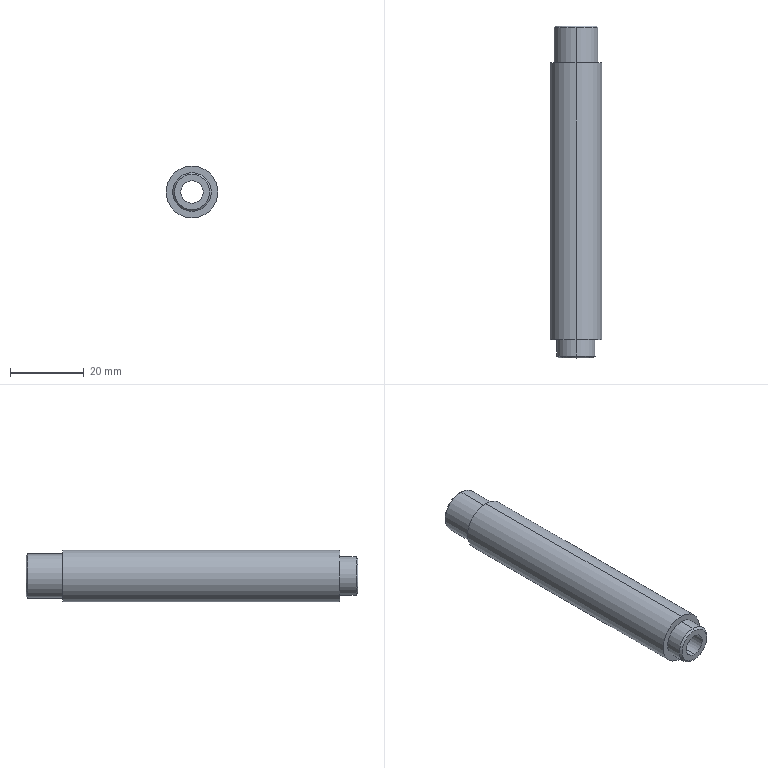Part | STEP file | 1 solid | 16 faces | box 14 x 90 x 14 mm | volume 10470 mm3 | cylinder 8 | cone 4 | plane 4 | commonest cylinder face diameters 6.1 x2 10.5 x2 12 x2 14 x2
STEP:
#1=CARTESIAN_POINT('',(0.,0.,0.));
#2=DIRECTION('',(0.,0.,1.));
#3=DIRECTION('',(1.,0.,0.));
#4=AXIS2_PLACEMENT_3D('',#1,#2,#3);
#5=CARTESIAN_POINT('',(0.,10.,5.5));
#6=VERTEX_POINT('',#5);
#7=CARTESIAN_POINT('',(0.,10.,-5.5));
#8=VERTEX_POINT('',#7);
#9=CARTESIAN_POINT('',(0.,10.,0.));
#10=DIRECTION('',(0.,1.,0.));
#11=DIRECTION('',(0.,0.,1.));
#12=AXIS2_PLACEMENT_3D('',#9,#10,#11);
#13=CIRCLE('',#12,5.5);
#14=CARTESIAN_POINT('',(0.,10.,0.));
#15=DIRECTION('',(0.,-1.,0.));
#16=DIRECTION('',(0.,0.,-1.));
#17=AXIS2_PLACEMENT_3D('',#14,#15,#16);
#18=CONICAL_SURFACE('',#17,5.5,0.7854);
#19=CARTESIAN_POINT('',(3.142,0.));
#20=DIRECTION('',(-1.,0.));
#21=VECTOR('',#20,1.);
#22=LINE('',#19,#21);
#23=(GEOMETRIC_REPRESENTATION_CONTEXT(2)PARAMETRIC_REPRESENTATION_CONTEXT()REPRESENTATION_CONTEXT('',''));
#24=DEFINITIONAL_REPRESENTATION('',(#22),#23);
#25=PCURVE('',#18,#24);
#26=CARTESIAN_POINT('',(0.,10.,0.));
#27=DIRECTION('',(0.,1.,0.));
#28=DIRECTION('',(0.,0.,1.));
#29=AXIS2_PLACEMENT_3D('',#26,#27,#28);
#30=PLANE('',#29);
#31=CARTESIAN_POINT('',(0.,0.));
#32=DIRECTION('',(1.,0.));
#33=AXIS2_PLACEMENT_2D('',#31,#32);
#34=CIRCLE('',#33,5.5);
#35=(GEOMETRIC_REPRESENTATION_CONTEXT(2)PARAMETRIC_REPRESENTATION_CONTEXT()REPRESENTATION_CONTEXT('',''));
#36=DEFINITIONAL_REPRESENTATION('',(#34),#35);
#37=PCURVE('',#30,#36);
#38=SURFACE_CURVE('',#13,(#25,#37),.PCURVE_S1.);
#39=EDGE_CURVE('',#6,#8,#38,.T.);
#40=ORIENTED_EDGE('',*,*,#39,.F.);
#41=CARTESIAN_POINT('',(0.,9.5,6.));
#42=VERTEX_POINT('',#41);
#43=CARTESIAN_POINT('',(0.,10.,5.5));
#44=DIRECTION('',(0.,-0.7071,0.7071));
#45=VECTOR('',#44,1.);
#46=LINE('',#43,#45);
#47=CARTESIAN_POINT('',(3.142,0.));
#48=DIRECTION('',(0.,1.));
#49=VECTOR('',#48,1.);
#50=LINE('',#47,#49);
#51=(GEOMETRIC_REPRESENTATION_CONTEXT(2)PARAMETRIC_REPRESENTATION_CONTEXT()REPRESENTATION_CONTEXT('',''));
#52=DEFINITIONAL_REPRESENTATION('',(#50),#51);
#53=PCURVE('',#18,#52);
#54=CARTESIAN_POINT('',(0.,10.,0.));
#55=DIRECTION('',(0.,-1.,0.));
#56=DIRECTION('',(0.,0.,-1.));
#57=AXIS2_PLACEMENT_3D('',#54,#55,#56);
#58=CONICAL_SURFACE('',#57,5.5,0.7854);
#59=CARTESIAN_POINT('',(3.142,0.));
#60=DIRECTION('',(0.,1.));
#61=VECTOR('',#60,1.);
#62=LINE('',#59,#61);
#63=(GEOMETRIC_REPRESENTATION_CONTEXT(2)PARAMETRIC_REPRESENTATION_CONTEXT()REPRESENTATION_CONTEXT('',''));
#64=DEFINITIONAL_REPRESENTATION('',(#62),#63);
#65=PCURVE('',#58,#64);
#66=SURFACE_CURVE('',#46,(#53,#65),.PCURVE_S1.);
#67=EDGE_CURVE('',#6,#42,#66,.T.);
#68=ORIENTED_EDGE('',*,*,#67,.T.);
#69=CARTESIAN_POINT('',(0.,9.5,-6.));
#70=VERTEX_POINT('',#69);
#71=CARTESIAN_POINT('',(0.,9.5,0.));
#72=DIRECTION('',(0.,-1.,0.));
#73=DIRECTION('',(0.,0.,1.));
#74=AXIS2_PLACEMENT_3D('',#71,#72,#73);
#75=CIRCLE('',#74,6.);
#76=CARTESIAN_POINT('',(-3.142,0.5));
#77=DIRECTION('',(1.,0.));
#78=VECTOR('',#77,1.);
#79=LINE('',#76,#78);
#80=(GEOMETRIC_REPRESENTATION_CONTEXT(2)PARAMETRIC_REPRESENTATION_CONTEXT()REPRESENTATION_CONTEXT('',''));
#81=DEFINITIONAL_REPRESENTATION('',(#79),#80);
#82=PCURVE('',#18,#81);
#83=CARTESIAN_POINT('',(0.,10.,0.));
#84=DIRECTION('',(0.,-1.,0.));
#85=DIRECTION('',(0.,0.,-1.));
#86=AXIS2_PLACEMENT_3D('',#83,#84,#85);
#87=CYLINDRICAL_SURFACE('',#86,6.);
#88=CARTESIAN_POINT('',(-3.142,0.5));
#89=DIRECTION('',(1.,0.));
#90=VECTOR('',#89,1.);
#91=LINE('',#88,#90);
#92=(GEOMETRIC_REPRESENTATION_CONTEXT(2)PARAMETRIC_REPRESENTATION_CONTEXT()REPRESENTATION_CONTEXT('',''));
#93=DEFINITIONAL_REPRESENTATION('',(#91),#92);
#94=PCURVE('',#87,#93);
#95=SURFACE_CURVE('',#75,(#82,#94),.PCURVE_S1.);
#96=EDGE_CURVE('',#70,#42,#95,.T.);
#97=ORIENTED_EDGE('',*,*,#96,.F.);
#98=CARTESIAN_POINT('',(0.,10.,-5.5));
#99=DIRECTION('',(0.,-0.7071,-0.7071));
#100=VECTOR('',#99,1.);
#101=LINE('',#98,#100);
#102=CARTESIAN_POINT('',(0.,0.));
#103=DIRECTION('',(0.,1.));
#104=VECTOR('',#103,1.);
#105=LINE('',#102,#104);
#106=(GEOMETRIC_REPRESENTATION_CONTEXT(2)PARAMETRIC_REPRESENTATION_CONTEXT()REPRESENTATION_CONTEXT('',''));
#107=DEFINITIONAL_REPRESENTATION('',(#105),#106);
#108=PCURVE('',#18,#107);
#109=CARTESIAN_POINT('',(6.283,0.));
#110=DIRECTION('',(0.,1.));
#111=VECTOR('',#110,1.);
#112=LINE('',#109,#111);
#113=(GEOMETRIC_REPRESENTATION_CONTEXT(2)PARAMETRIC_REPRESENTATION_CONTEXT()REPRESENTATION_CONTEXT('',''));
#114=DEFINITIONAL_REPRESENTATION('',(#112),#113);
#115=PCURVE('',#58,#114);
#116=SURFACE_CURVE('',#101,(#108,#115),.PCURVE_S1.);
#117=EDGE_CURVE('',#8,#70,#116,.T.);
#118=ORIENTED_EDGE('',*,*,#117,.F.);
#119=EDGE_LOOP('',(#40,#68,#97,#118));
#120=FACE_BOUND('',#119,.T.);
#121=ADVANCED_FACE('',(#120),#18,.T.);
#122=CARTESIAN_POINT('',(0.,-80.,-4.75));
#123=VERTEX_POINT('',#122);
#124=CARTESIAN_POINT('',(0.,-80.,4.75));
#125=VERTEX_POINT('',#124);
#126=CARTESIAN_POINT('',(0.,-80.,0.));
#127=DIRECTION('',(0.,-1.,0.));
#128=DIRECTION('',(0.,0.,1.));
#129=AXIS2_PLACEMENT_3D('',#126,#127,#128);
#130=CIRCLE('',#129,4.75);
#131=CARTESIAN_POINT('',(0.,-80.,0.));
#132=DIRECTION('',(0.,1.,0.));
#133=DIRECTION('',(0.,0.,1.));
#134=AXIS2_PLACEMENT_3D('',#131,#132,#133);
#135=CONICAL_SURFACE('',#134,4.75,0.7854);
#136=CARTESIAN_POINT('',(6.283,0.));
#137=DIRECTION('',(-1.,0.));
#138=VECTOR('',#137,1.);
#139=LINE('',#136,#138);
#140=(GEOMETRIC_REPRESENTATION_CONTEXT(2)PARAMETRIC_REPRESENTATION_CONTEXT()REPRESENTATION_CONTEXT('',''));
#141=DEFINITIONAL_REPRESENTATION('',(#139),#140);
#142=PCURVE('',#135,#141);
#143=CARTESIAN_POINT('',(0.,-80.,0.));
#144=DIRECTION('',(0.,1.,0.));
#145=DIRECTION('',(0.,0.,1.));
#146=AXIS2_PLACEMENT_3D('',#143,#144,#145);
#147=PLANE('',#146);
#148=CARTESIAN_POINT('',(4.75,0.));
#149=CARTESIAN_POINT('',(4.75,-8.227));
#150=CARTESIAN_POINT('',(-2.375,-4.114));
#151=CARTESIAN_POINT('',(-9.5,0.));
#152=CARTESIAN_POINT('',(-2.375,4.114));
#153=CARTESIAN_POINT('',(4.75,8.227));
#154=CARTESIAN_POINT('',(4.75,0.));
#155=(BOUNDED_CURVE()B_SPLINE_CURVE(2,(#148,#149,#150,#151,#152,#153,#154),.UNSPECIFIED.,.T.,.F.)B_SPLINE_CURVE_WITH_KNOTS((1,2,2,2,2,1),(-2.094,0.,2.094,4.189,6.283,8.378),.UNSPECIFIED.)CURVE()GEOMETRIC_REPRESENTATION_ITEM()RATIONAL_B_SPLINE_CURVE((1.,0.5,1.,0.5,1.,0.5,1.))REPRESENTATION_ITEM(''));
#156=(GEOMETRIC_REPRESENTATION_CONTEXT(2)PARAMETRIC_REPRESENTATION_CONTEXT()REPRESENTATION_CONTEXT('',''));
#157=DEFINITIONAL_REPRESENTATION('',(#155),#156);
#158=PCURVE('',#147,#157);
#159=SURFACE_CURVE('',#130,(#142,#158),.PCURVE_S1.);
#160=EDGE_CURVE('',#123,#125,#159,.T.);
#161=ORIENTED_EDGE('',*,*,#160,.F.);
#162=CARTESIAN_POINT('',(0.,-79.5,-5.25));
#163=VERTEX_POINT('',#162);
#164=CARTESIAN_POINT('',(0.,-80.,-4.75));
#165=DIRECTION('',(0.,0.7071,-0.7071));
#166=VECTOR('',#165,1.);
#167=LINE('',#164,#166);
#168=CARTESIAN_POINT('',(3.142,0.));
#169=DIRECTION('',(0.,1.));
#170=VECTOR('',#169,1.);
#171=LINE('',#168,#170);
#172=(GEOMETRIC_REPRESENTATION_CONTEXT(2)PARAMETRIC_REPRESENTATION_CONTEXT()REPRESENTATION_CONTEXT('',''));
#173=DEFINITIONAL_REPRESENTATION('',(#171),#172);
#174=PCURVE('',#135,#173);
#175=CARTESIAN_POINT('',(0.,-80.,0.));
#176=DIRECTION('',(0.,1.,0.));
#177=DIRECTION('',(0.,0.,1.));
#178=AXIS2_PLACEMENT_3D('',#175,#176,#177);
#179=CONICAL_SURFACE('',#178,4.75,0.7854);
#180=CARTESIAN_POINT('',(3.142,0.));
#181=DIRECTION('',(0.,1.));
#182=VECTOR('',#181,1.);
#183=LINE('',#180,#182);
#184=(GEOMETRIC_REPRESENTATION_CONTEXT(2)PARAMETRIC_REPRESENTATION_CONTEXT()REPRESENTATION_CONTEXT('',''));
#185=DEFINITIONAL_REPRESENTATION('',(#183),#184);
#186=PCURVE('',#179,#185);
#187=SURFACE_CURVE('',#167,(#174,#186),.PCURVE_S1.);
#188=EDGE_CURVE('',#123,#163,#187,.T.);
#189=ORIENTED_EDGE('',*,*,#188,.T.);
#190=CARTESIAN_POINT('',(0.,-79.5,5.25));
#191=VERTEX_POINT('',#190);
#192=CARTESIAN_POINT('',(0.,-79.5,0.));
#193=DIRECTION('',(0.,1.,0.));
#194=DIRECTION('',(0.,0.,1.));
#195=AXIS2_PLACEMENT_3D('',#192,#193,#194);
#196=CIRCLE('',#195,5.25);
#197=CARTESIAN_POINT('',(0.,0.5));
#198=DIRECTION('',(1.,0.));
#199=VECTOR('',#198,1.);
#200=LINE('',#197,#199);
#201=(GEOMETRIC_REPRESENTATION_CONTEXT(2)PARAMETRIC_REPRESENTATION_CONTEXT()REPRESENTATION_CONTEXT('',''));
#202=DEFINITIONAL_REPRESENTATION('',(#200),#201);
#203=PCURVE('',#135,#202);
#204=CARTESIAN_POINT('',(0.,-75.,0.));
#205=DIRECTION('',(0.,-1.,0.));
#206=DIRECTION('',(0.,0.,-1.));
#207=AXIS2_PLACEMENT_3D('',#204,#205,#206);
#208=CYLINDRICAL_SURFACE('',#207,5.25);
#209=CARTESIAN_POINT('',(3.142,4.5));
#210=DIRECTION('',(-1.,0.));
#211=VECTOR('',#210,1.);
#212=LINE('',#209,#211);
#213=(GEOMETRIC_REPRESENTATION_CONTEXT(2)PARAMETRIC_REPRESENTATION_CONTEXT()REPRESENTATION_CONTEXT('',''));
#214=DEFINITIONAL_REPRESENTATION('',(#212),#213);
#215=PCURVE('',#208,#214);
#216=SURFACE_CURVE('',#196,(#203,#215),.PCURVE_S1.);
#217=EDGE_CURVE('',#191,#163,#216,.T.);
#218=ORIENTED_EDGE('',*,*,#217,.F.);
#219=CARTESIAN_POINT('',(0.,-80.,4.75));
#220=DIRECTION('',(0.,0.7071,0.7071));
#221=VECTOR('',#220,1.);
#222=LINE('',#219,#221);
#223=CARTESIAN_POINT('',(0.,0.));
#224=DIRECTION('',(0.,1.));
#225=VECTOR('',#224,1.);
#226=LINE('',#223,#225);
#227=(GEOMETRIC_REPRESENTATION_CONTEXT(2)PARAMETRIC_REPRESENTATION_CONTEXT()REPRESENTATION_CONTEXT('',''));
#228=DEFINITIONAL_REPRESENTATION('',(#226),#227);
#229=PCURVE('',#135,#228);
#230=CARTESIAN_POINT('',(6.283,0.));
#231=DIRECTION('',(0.,1.));
#232=VECTOR('',#231,1.);
#233=LINE('',#230,#232);
#234=(GEOMETRIC_REPRESENTATION_CONTEXT(2)PARAMETRIC_REPRESENTATION_CONTEXT()REPRESENTATION_CONTEXT('',''));
#235=DEFINITIONAL_REPRESENTATION('',(#233),#234);
#236=PCURVE('',#179,#235);
#237=SURFACE_CURVE('',#222,(#229,#236),.PCURVE_S1.);
#238=EDGE_CURVE('',#125,#191,#237,.T.);
#239=ORIENTED_EDGE('',*,*,#238,.F.);
#240=EDGE_LOOP('',(#161,#189,#218,#239));
#241=FACE_BOUND('',#240,.T.);
#242=ADVANCED_FACE('',(#241),#135,.T.);
#243=CARTESIAN_POINT('',(0.,-75.,-5.25));
#244=VERTEX_POINT('',#243);
#245=CARTESIAN_POINT('',(0.,-75.,5.25));
#246=VERTEX_POINT('',#245);
#247=CARTESIAN_POINT('',(0.,-75.,0.));
#248=DIRECTION('',(0.,-1.,0.));
#249=DIRECTION('',(0.,0.,-1.));
#250=AXIS2_PLACEMENT_3D('',#247,#248,#249);
#251=CIRCLE('',#250,5.25);
#252=CARTESIAN_POINT('',(0.,0.));
#253=DIRECTION('',(1.,0.));
#254=VECTOR('',#253,1.);
#255=LINE('',#252,#254);
#256=(GEOMETRIC_REPRESENTATION_CONTEXT(2)PARAMETRIC_REPRESENTATION_CONTEXT()REPRESENTATION_CONTEXT('',''));
#257=DEFINITIONAL_REPRESENTATION('',(#255),#256);
#258=PCURVE('',#208,#257);
#259=CARTESIAN_POINT('',(0.,-75.,0.));
#260=DIRECTION('',(0.,-1.,0.));
#261=DIRECTION('',(0.,0.,-1.));
#262=AXIS2_PLACEMENT_3D('',#259,#260,#261);
#263=PLANE('',#262);
#264=CARTESIAN_POINT('',(0.,0.));
#265=DIRECTION('',(1.,0.));
#266=AXIS2_PLACEMENT_2D('',#264,#265);
#267=CIRCLE('',#266,5.25);
#268=(GEOMETRIC_REPRESENTATION_CONTEXT(2)PARAMETRIC_REPRESENTATION_CONTEXT()REPRESENTATION_CONTEXT('',''));
#269=DEFINITIONAL_REPRESENTATION('',(#267),#268);
#270=PCURVE('',#263,#269);
#271=SURFACE_CURVE('',#251,(#258,#270),.PCURVE_S1.);
#272=EDGE_CURVE('',#244,#246,#271,.T.);
#273=ORIENTED_EDGE('',*,*,#272,.T.);
#274=CARTESIAN_POINT('',(0.,-75.,5.25));
#275=DIRECTION('',(0.,-1.,0.));
#276=VECTOR('',#275,1.);
#277=LINE('',#274,#276);
#278=CARTESIAN_POINT('',(3.142,0.));
#279=DIRECTION('',(0.,1.));
#280=VECTOR('',#279,1.);
#281=LINE('',#278,#280);
#282=(GEOMETRIC_REPRESENTATION_CONTEXT(2)PARAMETRIC_REPRESENTATION_CONTEXT()REPRESENTATION_CONTEXT('',''));
#283=DEFINITIONAL_REPRESENTATION('',(#281),#282);
#284=PCURVE('',#208,#283);
#285=CARTESIAN_POINT('',(0.,-75.,0.));
#286=DIRECTION('',(0.,-1.,0.));
#287=DIRECTION('',(0.,0.,-1.));
#288=AXIS2_PLACEMENT_3D('',#285,#286,#287);
#289=CYLINDRICAL_SURFACE('',#288,5.25);
#290=CARTESIAN_POINT('',(3.142,0.));
#291=DIRECTION('',(0.,1.));
#292=VECTOR('',#291,1.);
#293=LINE('',#290,#292);
#294=(GEOMETRIC_REPRESENTATION_CONTEXT(2)PARAMETRIC_REPRESENTATION_CONTEXT()REPRESENTATION_CONTEXT('',''));
#295=DEFINITIONAL_REPRESENTATION('',(#293),#294);
#296=PCURVE('',#289,#295);
#297=SURFACE_CURVE('',#277,(#284,#296),.PCURVE_S1.);
#298=EDGE_CURVE('',#246,#191,#297,.T.);
#299=ORIENTED_EDGE('',*,*,#298,.T.);
#300=ORIENTED_EDGE('',*,*,#217,.T.);
#301=CARTESIAN_POINT('',(0.,-75.,-5.25));
#302=DIRECTION('',(0.,-1.,0.));
#303=VECTOR('',#302,1.);
#304=LINE('',#301,#303);
#305=CARTESIAN_POINT('',(0.,0.));
#306=DIRECTION('',(0.,1.));
#307=VECTOR('',#306,1.);
#308=LINE('',#305,#307);
#309=(GEOMETRIC_REPRESENTATION_CONTEXT(2)PARAMETRIC_REPRESENTATION_CONTEXT()REPRESENTATION_CONTEXT('',''));
#310=DEFINITIONAL_REPRESENTATION('',(#308),#309);
#311=PCURVE('',#208,#310);
#312=CARTESIAN_POINT('',(6.283,0.));
#313=DIRECTION('',(0.,1.));
#314=VECTOR('',#313,1.);
#315=LINE('',#312,#314);
#316=(GEOMETRIC_REPRESENTATION_CONTEXT(2)PARAMETRIC_REPRESENTATION_CONTEXT()REPRESENTATION_CONTEXT('',''));
#317=DEFINITIONAL_REPRESENTATION('',(#315),#316);
#318=PCURVE('',#289,#317);
#319=SURFACE_CURVE('',#304,(#311,#318),.PCURVE_S1.);
#320=EDGE_CURVE('',#244,#163,#319,.T.);
#321=ORIENTED_EDGE('',*,*,#320,.F.);
#322=EDGE_LOOP('',(#273,#299,#300,#321));
#323=FACE_BOUND('',#322,.T.);
#324=ADVANCED_FACE('',(#323),#208,.T.);
#325=ORIENTED_EDGE('',*,*,#96,.T.);
#326=CARTESIAN_POINT('',(0.,0.,6.));
#327=VERTEX_POINT('',#326);
#328=CARTESIAN_POINT('',(0.,10.,6.));
#329=DIRECTION('',(0.,-1.,0.));
#330=VECTOR('',#329,1.);
#331=LINE('',#328,#330);
#332=CARTESIAN_POINT('',(3.142,0.));
#333=DIRECTION('',(0.,1.));
#334=VECTOR('',#333,1.);
#335=LINE('',#332,#334);
#336=(GEOMETRIC_REPRESENTATION_CONTEXT(2)PARAMETRIC_REPRESENTATION_CONTEXT()REPRESENTATION_CONTEXT('',''));
#337=DEFINITIONAL_REPRESENTATION('',(#335),#336);
#338=PCURVE('',#87,#337);
#339=CARTESIAN_POINT('',(0.,10.,0.));
#340=DIRECTION('',(0.,-1.,0.));
#341=DIRECTION('',(0.,0.,-1.));
#342=AXIS2_PLACEMENT_3D('',#339,#340,#341);
#343=CYLINDRICAL_SURFACE('',#342,6.);
#344=CARTESIAN_POINT('',(3.142,0.));
#345=DIRECTION('',(0.,1.));
#346=VECTOR('',#345,1.);
#347=LINE('',#344,#346);
#348=(GEOMETRIC_REPRESENTATION_CONTEXT(2)PARAMETRIC_REPRESENTATION_CONTEXT()REPRESENTATION_CONTEXT('',''));
#349=DEFINITIONAL_REPRESENTATION('',(#347),#348);
#350=PCURVE('',#343,#349);
#351=SURFACE_CURVE('',#331,(#338,#350),.PCURVE_S1.);
#352=EDGE_CURVE('',#42,#327,#351,.T.);
#353=ORIENTED_EDGE('',*,*,#352,.T.);
#354=CARTESIAN_POINT('',(0.,0.,-6.));
#355=VERTEX_POINT('',#354);
#356=CARTESIAN_POINT('',(0.,0.,0.));
#357=DIRECTION('',(0.,1.,0.));
#358=DIRECTION('',(0.,0.,1.));
#359=AXIS2_PLACEMENT_3D('',#356,#357,#358);
#360=CIRCLE('',#359,6.);
#361=CARTESIAN_POINT('',(3.142,10.));
#362=DIRECTION('',(-1.,0.));
#363=VECTOR('',#362,1.);
#364=LINE('',#361,#363);
#365=(GEOMETRIC_REPRESENTATION_CONTEXT(2)PARAMETRIC_REPRESENTATION_CONTEXT()REPRESENTATION_CONTEXT('',''));
#366=DEFINITIONAL_REPRESENTATION('',(#364),#365);
#367=PCURVE('',#87,#366);
#368=CARTESIAN_POINT('',(0.,0.,0.));
#369=DIRECTION('',(0.,1.,0.));
#370=DIRECTION('',(0.,0.,1.));
#371=AXIS2_PLACEMENT_3D('',#368,#369,#370);
#372=PLANE('',#371);
#373=CARTESIAN_POINT('',(0.,0.));
#374=DIRECTION('',(1.,0.));
#375=AXIS2_PLACEMENT_2D('',#373,#374);
#376=CIRCLE('',#375,6.);
#377=(GEOMETRIC_REPRESENTATION_CONTEXT(2)PARAMETRIC_REPRESENTATION_CONTEXT()REPRESENTATION_CONTEXT('',''));
#378=DEFINITIONAL_REPRESENTATION('',(#376),#377);
#379=PCURVE('',#372,#378);
#380=SURFACE_CURVE('',#360,(#367,#379),.PCURVE_S1.);
#381=EDGE_CURVE('',#327,#355,#380,.T.);
#382=ORIENTED_EDGE('',*,*,#381,.T.);
#383=CARTESIAN_POINT('',(0.,10.,-6.));
#384=DIRECTION('',(0.,-1.,0.));
#385=VECTOR('',#384,1.);
#386=LINE('',#383,#385);
#387=CARTESIAN_POINT('',(0.,0.));
#388=DIRECTION('',(0.,1.));
#389=VECTOR('',#388,1.);
#390=LINE('',#387,#389);
#391=(GEOMETRIC_REPRESENTATION_CONTEXT(2)PARAMETRIC_REPRESENTATION_CONTEXT()REPRESENTATION_CONTEXT('',''));
#392=DEFINITIONAL_REPRESENTATION('',(#390),#391);
#393=PCURVE('',#87,#392);
#394=CARTESIAN_POINT('',(6.283,0.));
#395=DIRECTION('',(0.,1.));
#396=VECTOR('',#395,1.);
#397=LINE('',#394,#396);
#398=(GEOMETRIC_REPRESENTATION_CONTEXT(2)PARAMETRIC_REPRESENTATION_CONTEXT()REPRESENTATION_CONTEXT('',''));
#399=DEFINITIONAL_REPRESENTATION('',(#397),#398);
#400=PCURVE('',#343,#399);
#401=SURFACE_CURVE('',#386,(#393,#400),.PCURVE_S1.);
#402=EDGE_CURVE('',#70,#355,#401,.T.);
#403=ORIENTED_EDGE('',*,*,#402,.F.);
#404=EDGE_LOOP('',(#325,#353,#382,#403));
#405=FACE_BOUND('',#404,.T.);
#406=ADVANCED_FACE('',(#405),#87,.T.);
#407=CARTESIAN_POINT('',(0.,-80.,3.05));
#408=VERTEX_POINT('',#407);
#409=CARTESIAN_POINT('',(0.,10.,3.05));
#410=VERTEX_POINT('',#409);
#411=CARTESIAN_POINT('',(0.,-80.,3.05));
#412=DIRECTION('',(0.,1.,0.));
#413=VECTOR('',#412,1.);
#414=LINE('',#411,#413);
#415=CARTESIAN_POINT('',(0.,-80.,0.));
#416=DIRECTION('',(0.,1.,0.));
#417=DIRECTION('',(0.,0.,1.));
#418=AXIS2_PLACEMENT_3D('',#415,#416,#417);
#419=CYLINDRICAL_SURFACE('',#418,3.05);
#420=CARTESIAN_POINT('',(6.283,0.));
#421=DIRECTION('',(0.,1.));
#422=VECTOR('',#421,1.);
#423=LINE('',#420,#422);
#424=(GEOMETRIC_REPRESENTATION_CONTEXT(2)PARAMETRIC_REPRESENTATION_CONTEXT()REPRESENTATION_CONTEXT('',''));
#425=DEFINITIONAL_REPRESENTATION('',(#423),#424);
#426=PCURVE('',#419,#425);
#427=CARTESIAN_POINT('',(0.,-80.,0.));
#428=DIRECTION('',(0.,1.,0.));
#429=DIRECTION('',(0.,0.,1.));
#430=AXIS2_PLACEMENT_3D('',#427,#428,#429);
#431=CYLINDRICAL_SURFACE('',#430,3.05);
#432=CARTESIAN_POINT('',(0.,0.));
#433=DIRECTION('',(0.,1.));
#434=VECTOR('',#433,1.);
#435=LINE('',#432,#434);
#436=(GEOMETRIC_REPRESENTATION_CONTEXT(2)PARAMETRIC_REPRESENTATION_CONTEXT()REPRESENTATION_CONTEXT('',''));
#437=DEFINITIONAL_REPRESENTATION('',(#435),#436);
#438=PCURVE('',#431,#437);
#439=SURFACE_CURVE('',#414,(#426,#438),.PCURVE_S1.);
#440=EDGE_CURVE('',#408,#410,#439,.T.);
#441=ORIENTED_EDGE('',*,*,#440,.T.);
#442=CARTESIAN_POINT('',(0.,10.,-3.05));
#443=VERTEX_POINT('',#442);
#444=CARTESIAN_POINT('',(0.,10.,0.));
#445=DIRECTION('',(0.,1.,0.));
#446=DIRECTION('',(0.,0.,1.));
#447=AXIS2_PLACEMENT_3D('',#444,#445,#446);
#448=CIRCLE('',#447,3.05);
#449=CARTESIAN_POINT('',(0.,90.));
#450=DIRECTION('',(1.,0.));
#451=VECTOR('',#450,1.);
#452=LINE('',#449,#451);
#453=(GEOMETRIC_REPRESENTATION_CONTEXT(2)PARAMETRIC_REPRESENTATION_CONTEXT()REPRESENTATION_CONTEXT('',''));
#454=DEFINITIONAL_REPRESENTATION('',(#452),#453);
#455=PCURVE('',#419,#454);
#456=CARTESIAN_POINT('',(0.,0.));
#457=DIRECTION('',(1.,0.));
#458=AXIS2_PLACEMENT_2D('',#456,#457);
#459=CIRCLE('',#458,3.05);
#460=(GEOMETRIC_REPRESENTATION_CONTEXT(2)PARAMETRIC_REPRESENTATION_CONTEXT()REPRESENTATION_CONTEXT('',''));
#461=DEFINITIONAL_REPRESENTATION('',(#459),#460);
#462=PCURVE('',#30,#461);
#463=SURFACE_CURVE('',#448,(#455,#462),.PCURVE_S1.);
#464=EDGE_CURVE('',#443,#410,#463,.T.);
#465=ORIENTED_EDGE('',*,*,#464,.F.);
#466=CARTESIAN_POINT('',(0.,-80.,-3.05));
#467=VERTEX_POINT('',#466);
#468=CARTESIAN_POINT('',(0.,-80.,-3.05));
#469=DIRECTION('',(0.,1.,0.));
#470=VECTOR('',#469,1.);
#471=LINE('',#468,#470);
#472=CARTESIAN_POINT('',(3.142,0.));
#473=DIRECTION('',(0.,1.));
#474=VECTOR('',#473,1.);
#475=LINE('',#472,#474);
#476=(GEOMETRIC_REPRESENTATION_CONTEXT(2)PARAMETRIC_REPRESENTATION_CONTEXT()REPRESENTATION_CONTEXT('',''));
#477=DEFINITIONAL_REPRESENTATION('',(#475),#476);
#478=PCURVE('',#419,#477);
#479=CARTESIAN_POINT('',(3.142,0.));
#480=DIRECTION('',(0.,1.));
#481=VECTOR('',#480,1.);
#482=LINE('',#479,#481);
#483=(GEOMETRIC_REPRESENTATION_CONTEXT(2)PARAMETRIC_REPRESENTATION_CONTEXT()REPRESENTATION_CONTEXT('',''));
#484=DEFINITIONAL_REPRESENTATION('',(#482),#483);
#485=PCURVE('',#431,#484);
#486=SURFACE_CURVE('',#471,(#478,#485),.PCURVE_S1.);
#487=EDGE_CURVE('',#467,#443,#486,.T.);
#488=ORIENTED_EDGE('',*,*,#487,.F.);
#489=CARTESIAN_POINT('',(0.,-80.,0.));
#490=DIRECTION('',(0.,1.,0.));
#491=DIRECTION('',(0.,0.,1.));
#492=AXIS2_PLACEMENT_3D('',#489,#490,#491);
#493=CIRCLE('',#492,3.05);
#494=CARTESIAN_POINT('',(0.,0.));
#495=DIRECTION('',(1.,0.));
#496=VECTOR('',#495,1.);
#497=LINE('',#494,#496);
#498=(GEOMETRIC_REPRESENTATION_CONTEXT(2)PARAMETRIC_REPRESENTATION_CONTEXT()REPRESENTATION_CONTEXT('',''));
#499=DEFINITIONAL_REPRESENTATION('',(#497),#498);
#500=PCURVE('',#419,#499);
#501=CARTESIAN_POINT('',(0.,0.));
#502=DIRECTION('',(1.,0.));
#503=AXIS2_PLACEMENT_2D('',#501,#502);
#504=CIRCLE('',#503,3.05);
#505=(GEOMETRIC_REPRESENTATION_CONTEXT(2)PARAMETRIC_REPRESENTATION_CONTEXT()REPRESENTATION_CONTEXT('',''));
#506=DEFINITIONAL_REPRESENTATION('',(#504),#505);
#507=PCURVE('',#147,#506);
#508=SURFACE_CURVE('',#493,(#500,#507),.PCURVE_S1.);
#509=EDGE_CURVE('',#467,#408,#508,.T.);
#510=ORIENTED_EDGE('',*,*,#509,.T.);
#511=EDGE_LOOP('',(#441,#465,#488,#510));
#512=FACE_BOUND('',#511,.F.);
#513=ADVANCED_FACE('',(#512),#419,.F.);
#514=CARTESIAN_POINT('',(0.,-75.,-7.));
#515=VERTEX_POINT('',#514);
#516=CARTESIAN_POINT('',(0.,-75.,7.));
#517=VERTEX_POINT('',#516);
#518=CARTESIAN_POINT('',(0.,-75.,0.));
#519=DIRECTION('',(0.,-1.,0.));
#520=DIRECTION('',(0.,0.,-1.));
#521=AXIS2_PLACEMENT_3D('',#518,#519,#520);
#522=CIRCLE('',#521,7.);
#523=CARTESIAN_POINT('',(0.,-80.,0.));
#524=DIRECTION('',(0.,1.,0.));
#525=DIRECTION('',(0.,0.,1.));
#526=AXIS2_PLACEMENT_3D('',#523,#524,#525);
#527=CYLINDRICAL_SURFACE('',#526,7.);
#528=CARTESIAN_POINT('',(3.142,5.));
#529=DIRECTION('',(-1.,0.));
#530=VECTOR('',#529,1.);
#531=LINE('',#528,#530);
#532=(GEOMETRIC_REPRESENTATION_CONTEXT(2)PARAMETRIC_REPRESENTATION_CONTEXT()REPRESENTATION_CONTEXT('',''));
#533=DEFINITIONAL_REPRESENTATION('',(#531),#532);
#534=PCURVE('',#527,#533);
#535=CARTESIAN_POINT('',(0.,0.));
#536=DIRECTION('',(1.,0.));
#537=AXIS2_PLACEMENT_2D('',#535,#536);
#538=CIRCLE('',#537,7.);
#539=(GEOMETRIC_REPRESENTATION_CONTEXT(2)PARAMETRIC_REPRESENTATION_CONTEXT()REPRESENTATION_CONTEXT('',''));
#540=DEFINITIONAL_REPRESENTATION('',(#538),#539);
#541=PCURVE('',#263,#540);
#542=SURFACE_CURVE('',#522,(#534,#541),.PCURVE_S1.);
#543=EDGE_CURVE('',#515,#517,#542,.T.);
#544=ORIENTED_EDGE('',*,*,#543,.F.);
#545=CARTESIAN_POINT('',(0.,0.,-7.));
#546=VERTEX_POINT('',#545);
#547=CARTESIAN_POINT('',(0.,-80.,-7.));
#548=DIRECTION('',(0.,1.,0.));
#549=VECTOR('',#548,1.);
#550=LINE('',#547,#549);
#551=CARTESIAN_POINT('',(3.142,0.));
#552=DIRECTION('',(0.,1.));
#553=VECTOR('',#552,1.);
#554=LINE('',#551,#553);
#555=(GEOMETRIC_REPRESENTATION_CONTEXT(2)PARAMETRIC_REPRESENTATION_CONTEXT()REPRESENTATION_CONTEXT('',''));
#556=DEFINITIONAL_REPRESENTATION('',(#554),#555);
#557=PCURVE('',#527,#556);
#558=CARTESIAN_POINT('',(0.,-80.,0.));
#559=DIRECTION('',(0.,1.,0.));
#560=DIRECTION('',(0.,0.,1.));
#561=AXIS2_PLACEMENT_3D('',#558,#559,#560);
#562=CYLINDRICAL_SURFACE('',#561,7.);
#563=CARTESIAN_POINT('',(3.142,0.));
#564=DIRECTION('',(0.,1.));
#565=VECTOR('',#564,1.);
#566=LINE('',#563,#565);
#567=(GEOMETRIC_REPRESENTATION_CONTEXT(2)PARAMETRIC_REPRESENTATION_CONTEXT()REPRESENTATION_CONTEXT('',''));
#568=DEFINITIONAL_REPRESENTATION('',(#566),#567);
#569=PCURVE('',#562,#568);
#570=SURFACE_CURVE('',#550,(#557,#569),.PCURVE_S1.);
#571=EDGE_CURVE('',#515,#546,#570,.T.);
#572=ORIENTED_EDGE('',*,*,#571,.T.);
#573=CARTESIAN_POINT('',(0.,0.,7.));
#574=VERTEX_POINT('',#573);
#575=CARTESIAN_POINT('',(0.,0.,0.));
#576=DIRECTION('',(0.,1.,0.));
#577=DIRECTION('',(0.,0.,1.));
#578=AXIS2_PLACEMENT_3D('',#575,#576,#577);
#579=CIRCLE('',#578,7.);
#580=CARTESIAN_POINT('',(0.,80.));
#581=DIRECTION('',(1.,0.));
#582=VECTOR('',#581,1.);
#583=LINE('',#580,#582);
#584=(GEOMETRIC_REPRESENTATION_CONTEXT(2)PARAMETRIC_REPRESENTATION_CONTEXT()REPRESENTATION_CONTEXT('',''));
#585=DEFINITIONAL_REPRESENTATION('',(#583),#584);
#586=PCURVE('',#527,#585);
#587=CARTESIAN_POINT('',(0.,0.));
#588=DIRECTION('',(1.,0.));
#589=AXIS2_PLACEMENT_2D('',#587,#588);
#590=CIRCLE('',#589,7.);
#591=(GEOMETRIC_REPRESENTATION_CONTEXT(2)PARAMETRIC_REPRESENTATION_CONTEXT()REPRESENTATION_CONTEXT('',''));
#592=DEFINITIONAL_REPRESENTATION('',(#590),#591);
#593=PCURVE('',#372,#592);
#594=SURFACE_CURVE('',#579,(#586,#593),.PCURVE_S1.);
#595=EDGE_CURVE('',#574,#546,#594,.T.);
#596=ORIENTED_EDGE('',*,*,#595,.F.);
#597=CARTESIAN_POINT('',(0.,-80.,7.));
#598=DIRECTION('',(0.,1.,0.));
#599=VECTOR('',#598,1.);
#600=LINE('',#597,#599);
#601=CARTESIAN_POINT('',(0.,0.));
#602=DIRECTION('',(0.,1.));
#603=VECTOR('',#602,1.);
#604=LINE('',#601,#603);
#605=(GEOMETRIC_REPRESENTATION_CONTEXT(2)PARAMETRIC_REPRESENTATION_CONTEXT()REPRESENTATION_CONTEXT('',''));
#606=DEFINITIONAL_REPRESENTATION('',(#604),#605);
#607=PCURVE('',#527,#606);
#608=CARTESIAN_POINT('',(6.283,0.));
#609=DIRECTION('',(0.,1.));
#610=VECTOR('',#609,1.);
#611=LINE('',#608,#610);
#612=(GEOMETRIC_REPRESENTATION_CONTEXT(2)PARAMETRIC_REPRESENTATION_CONTEXT()REPRESENTATION_CONTEXT('',''));
#613=DEFINITIONAL_REPRESENTATION('',(#611),#612);
#614=PCURVE('',#562,#613);
#615=SURFACE_CURVE('',#600,(#607,#614),.PCURVE_S1.);
#616=EDGE_CURVE('',#517,#574,#615,.T.);
#617=ORIENTED_EDGE('',*,*,#616,.F.);
#618=EDGE_LOOP('',(#544,#572,#596,#617));
#619=FACE_BOUND('',#618,.T.);
#620=ADVANCED_FACE('',(#619),#527,.T.);
#621=ORIENTED_EDGE('',*,*,#571,.F.);
#622=CARTESIAN_POINT('',(0.,-75.,0.));
#623=DIRECTION('',(0.,-1.,0.));
#624=DIRECTION('',(0.,0.,-1.));
#625=AXIS2_PLACEMENT_3D('',#622,#623,#624);
#626=CIRCLE('',#625,7.);
#627=CARTESIAN_POINT('',(9.425,5.));
#628=DIRECTION('',(-1.,0.));
#629=VECTOR('',#628,1.);
#630=LINE('',#627,#629);
#631=(GEOMETRIC_REPRESENTATION_CONTEXT(2)PARAMETRIC_REPRESENTATION_CONTEXT()REPRESENTATION_CONTEXT('',''));
#632=DEFINITIONAL_REPRESENTATION('',(#630),#631);
#633=PCURVE('',#562,#632);
#634=CARTESIAN_POINT('',(0.,0.));
#635=DIRECTION('',(1.,0.));
#636=AXIS2_PLACEMENT_2D('',#634,#635);
#637=CIRCLE('',#636,7.);
#638=(GEOMETRIC_REPRESENTATION_CONTEXT(2)PARAMETRIC_REPRESENTATION_CONTEXT()REPRESENTATION_CONTEXT('',''));
#639=DEFINITIONAL_REPRESENTATION('',(#637),#638);
#640=PCURVE('',#263,#639);
#641=SURFACE_CURVE('',#626,(#633,#640),.PCURVE_S1.);
#642=EDGE_CURVE('',#517,#515,#641,.T.);
#643=ORIENTED_EDGE('',*,*,#642,.F.);
#644=ORIENTED_EDGE('',*,*,#616,.T.);
#645=CARTESIAN_POINT('',(0.,0.,0.));
#646=DIRECTION('',(0.,1.,0.));
#647=DIRECTION('',(0.,0.,1.));
#648=AXIS2_PLACEMENT_3D('',#645,#646,#647);
#649=CIRCLE('',#648,7.);
#650=CARTESIAN_POINT('',(0.,80.));
#651=DIRECTION('',(1.,0.));
#652=VECTOR('',#651,1.);
#653=LINE('',#650,#652);
#654=(GEOMETRIC_REPRESENTATION_CONTEXT(2)PARAMETRIC_REPRESENTATION_CONTEXT()REPRESENTATION_CONTEXT('',''));
#655=DEFINITIONAL_REPRESENTATION('',(#653),#654);
#656=PCURVE('',#562,#655);
#657=CARTESIAN_POINT('',(0.,0.));
#658=DIRECTION('',(1.,0.));
#659=AXIS2_PLACEMENT_2D('',#657,#658);
#660=CIRCLE('',#659,7.);
#661=(GEOMETRIC_REPRESENTATION_CONTEXT(2)PARAMETRIC_REPRESENTATION_CONTEXT()REPRESENTATION_CONTEXT('',''));
#662=DEFINITIONAL_REPRESENTATION('',(#660),#661);
#663=PCURVE('',#372,#662);
#664=SURFACE_CURVE('',#649,(#656,#663),.PCURVE_S1.);
#665=EDGE_CURVE('',#546,#574,#664,.T.);
#666=ORIENTED_EDGE('',*,*,#665,.F.);
#667=EDGE_LOOP('',(#621,#643,#644,#666));
#668=FACE_BOUND('',#667,.T.);
#669=ADVANCED_FACE('',(#668),#562,.T.);
#670=CARTESIAN_POINT('',(0.,-80.,0.));
#671=DIRECTION('',(0.,-1.,0.));
#672=DIRECTION('',(0.,0.,1.));
#673=AXIS2_PLACEMENT_3D('',#670,#671,#672);
#674=CIRCLE('',#673,4.75);
#675=CARTESIAN_POINT('',(4.75,0.));
#676=CARTESIAN_POINT('',(4.75,-8.227));
#677=CARTESIAN_POINT('',(-2.375,-4.114));
#678=CARTESIAN_POINT('',(-9.5,0.));
#679=CARTESIAN_POINT('',(-2.375,4.114));
#680=CARTESIAN_POINT('',(4.75,8.227));
#681=CARTESIAN_POINT('',(4.75,0.));
#682=(BOUNDED_CURVE()B_SPLINE_CURVE(2,(#675,#676,#677,#678,#679,#680,#681),.UNSPECIFIED.,.T.,.F.)B_SPLINE_CURVE_WITH_KNOTS((1,2,2,2,2,1),(-2.094,0.,2.094,4.189,6.283,8.378),.UNSPECIFIED.)CURVE()GEOMETRIC_REPRESENTATION_ITEM()RATIONAL_B_SPLINE_CURVE((1.,0.5,1.,0.5,1.,0.5,1.))REPRESENTATION_ITEM(''));
#683=(GEOMETRIC_REPRESENTATION_CONTEXT(2)PARAMETRIC_REPRESENTATION_CONTEXT()REPRESENTATION_CONTEXT('',''));
#684=DEFINITIONAL_REPRESENTATION('',(#682),#683);
#685=PCURVE('',#147,#684);
#686=CARTESIAN_POINT('',(6.283,0.));
#687=DIRECTION('',(-1.,0.));
#688=VECTOR('',#687,1.);
#689=LINE('',#686,#688);
#690=(GEOMETRIC_REPRESENTATION_CONTEXT(2)PARAMETRIC_REPRESENTATION_CONTEXT()REPRESENTATION_CONTEXT('',''));
#691=DEFINITIONAL_REPRESENTATION('',(#689),#690);
#692=PCURVE('',#179,#691);
#693=SURFACE_CURVE('',#674,(#685,#692),.PCURVE_S1.);
#694=EDGE_CURVE('',#125,#123,#693,.T.);
#695=ORIENTED_EDGE('',*,*,#694,.T.);
#696=ORIENTED_EDGE('',*,*,#160,.T.);
#697=EDGE_LOOP('',(#695,#696));
#698=FACE_BOUND('',#697,.T.);
#699=CARTESIAN_POINT('',(0.,-80.,0.));
#700=DIRECTION('',(0.,1.,0.));
#701=DIRECTION('',(0.,0.,1.));
#702=AXIS2_PLACEMENT_3D('',#699,#700,#701);
#703=CIRCLE('',#702,3.05);
#704=CARTESIAN_POINT('',(0.,0.));
#705=DIRECTION('',(1.,0.));
#706=AXIS2_PLACEMENT_2D('',#704,#705);
#707=CIRCLE('',#706,3.05);
#708=(GEOMETRIC_REPRESENTATION_CONTEXT(2)PARAMETRIC_REPRESENTATION_CONTEXT()REPRESENTATION_CONTEXT('',''));
#709=DEFINITIONAL_REPRESENTATION('',(#707),#708);
#710=PCURVE('',#147,#709);
#711=CARTESIAN_POINT('',(0.,0.));
#712=DIRECTION('',(1.,0.));
#713=VECTOR('',#712,1.);
#714=LINE('',#711,#713);
#715=(GEOMETRIC_REPRESENTATION_CONTEXT(2)PARAMETRIC_REPRESENTATION_CONTEXT()REPRESENTATION_CONTEXT('',''));
#716=DEFINITIONAL_REPRESENTATION('',(#714),#715);
#717=PCURVE('',#431,#716);
#718=SURFACE_CURVE('',#703,(#710,#717),.PCURVE_S1.);
#719=EDGE_CURVE('',#408,#467,#718,.T.);
#720=ORIENTED_EDGE('',*,*,#719,.T.);
#721=ORIENTED_EDGE('',*,*,#509,.T.);
#722=EDGE_LOOP('',(#720,#721));
#723=FACE_BOUND('',#722,.T.);
#724=ADVANCED_FACE('',(#698,#723),#147,.F.);
#725=CARTESIAN_POINT('',(0.,0.,0.));
#726=DIRECTION('',(0.,1.,0.));
#727=DIRECTION('',(0.,0.,1.));
#728=AXIS2_PLACEMENT_3D('',#725,#726,#727);
#729=CIRCLE('',#728,6.);
#730=CARTESIAN_POINT('',(0.,0.));
#731=DIRECTION('',(1.,0.));
#732=AXIS2_PLACEMENT_2D('',#730,#731);
#733=CIRCLE('',#732,6.);
#734=(GEOMETRIC_REPRESENTATION_CONTEXT(2)PARAMETRIC_REPRESENTATION_CONTEXT()REPRESENTATION_CONTEXT('',''));
#735=DEFINITIONAL_REPRESENTATION('',(#733),#734);
#736=PCURVE('',#372,#735);
#737=CARTESIAN_POINT('',(9.425,10.));
#738=DIRECTION('',(-1.,0.));
#739=VECTOR('',#738,1.);
#740=LINE('',#737,#739);
#741=(GEOMETRIC_REPRESENTATION_CONTEXT(2)PARAMETRIC_REPRESENTATION_CONTEXT()REPRESENTATION_CONTEXT('',''));
#742=DEFINITIONAL_REPRESENTATION('',(#740),#741);
#743=PCURVE('',#343,#742);
#744=SURFACE_CURVE('',#729,(#736,#743),.PCURVE_S1.);
#745=EDGE_CURVE('',#355,#327,#744,.T.);
#746=ORIENTED_EDGE('',*,*,#745,.F.);
#747=ORIENTED_EDGE('',*,*,#381,.F.);
#748=EDGE_LOOP('',(#746,#747));
#749=FACE_BOUND('',#748,.T.);
#750=ORIENTED_EDGE('',*,*,#595,.T.);
#751=ORIENTED_EDGE('',*,*,#665,.T.);
#752=EDGE_LOOP('',(#750,#751));
#753=FACE_BOUND('',#752,.T.);
#754=ADVANCED_FACE('',(#749,#753),#372,.T.);
#755=CARTESIAN_POINT('',(0.,10.,0.));
#756=DIRECTION('',(0.,1.,0.));
#757=DIRECTION('',(0.,0.,1.));
#758=AXIS2_PLACEMENT_3D('',#755,#756,#757);
#759=CIRCLE('',#758,3.05);
#760=CARTESIAN_POINT('',(0.,90.));
#761=DIRECTION('',(1.,0.));
#762=VECTOR('',#761,1.);
#763=LINE('',#760,#762);
#764=(GEOMETRIC_REPRESENTATION_CONTEXT(2)PARAMETRIC_REPRESENTATION_CONTEXT()REPRESENTATION_CONTEXT('',''));
#765=DEFINITIONAL_REPRESENTATION('',(#763),#764);
#766=PCURVE('',#431,#765);
#767=CARTESIAN_POINT('',(0.,0.));
#768=DIRECTION('',(1.,0.));
#769=AXIS2_PLACEMENT_2D('',#767,#768);
#770=CIRCLE('',#769,3.05);
#771=(GEOMETRIC_REPRESENTATION_CONTEXT(2)PARAMETRIC_REPRESENTATION_CONTEXT()REPRESENTATION_CONTEXT('',''));
#772=DEFINITIONAL_REPRESENTATION('',(#770),#771);
#773=PCURVE('',#30,#772);
#774=SURFACE_CURVE('',#759,(#766,#773),.PCURVE_S1.);
#775=EDGE_CURVE('',#410,#443,#774,.T.);
#776=ORIENTED_EDGE('',*,*,#775,.F.);
#777=ORIENTED_EDGE('',*,*,#440,.F.);
#778=ORIENTED_EDGE('',*,*,#719,.T.);
#779=ORIENTED_EDGE('',*,*,#487,.T.);
#780=EDGE_LOOP('',(#776,#777,#778,#779));
#781=FACE_BOUND('',#780,.F.);
#782=ADVANCED_FACE('',(#781),#431,.F.);
#783=CARTESIAN_POINT('',(0.,10.,0.));
#784=DIRECTION('',(0.,1.,0.));
#785=DIRECTION('',(0.,0.,1.));
#786=AXIS2_PLACEMENT_3D('',#783,#784,#785);
#787=CIRCLE('',#786,5.5);
#788=CARTESIAN_POINT('',(0.,0.));
#789=DIRECTION('',(1.,0.));
#790=AXIS2_PLACEMENT_2D('',#788,#789);
#791=CIRCLE('',#790,5.5);
#792=(GEOMETRIC_REPRESENTATION_CONTEXT(2)PARAMETRIC_REPRESENTATION_CONTEXT()REPRESENTATION_CONTEXT('',''));
#793=DEFINITIONAL_REPRESENTATION('',(#791),#792);
#794=PCURVE('',#30,#793);
#795=CARTESIAN_POINT('',(9.425,0.));
#796=DIRECTION('',(-1.,0.));
#797=VECTOR('',#796,1.);
#798=LINE('',#795,#797);
#799=(GEOMETRIC_REPRESENTATION_CONTEXT(2)PARAMETRIC_REPRESENTATION_CONTEXT()REPRESENTATION_CONTEXT('',''));
#800=DEFINITIONAL_REPRESENTATION('',(#798),#799);
#801=PCURVE('',#58,#800);
#802=SURFACE_CURVE('',#787,(#794,#801),.PCURVE_S1.);
#803=EDGE_CURVE('',#8,#6,#802,.T.);
#804=ORIENTED_EDGE('',*,*,#803,.T.);
#805=ORIENTED_EDGE('',*,*,#39,.T.);
#806=EDGE_LOOP('',(#804,#805));
#807=FACE_BOUND('',#806,.T.);
#808=ORIENTED_EDGE('',*,*,#775,.F.);
#809=ORIENTED_EDGE('',*,*,#464,.F.);
#810=EDGE_LOOP('',(#808,#809));
#811=FACE_BOUND('',#810,.T.);
#812=ADVANCED_FACE('',(#807,#811),#30,.T.);
#813=ORIENTED_EDGE('',*,*,#352,.F.);
#814=CARTESIAN_POINT('',(0.,9.5,0.));
#815=DIRECTION('',(0.,-1.,0.));
#816=DIRECTION('',(0.,0.,1.));
#817=AXIS2_PLACEMENT_3D('',#814,#815,#816);
#818=CIRCLE('',#817,6.);
#819=CARTESIAN_POINT('',(3.142,0.5));
#820=DIRECTION('',(1.,0.));
#821=VECTOR('',#820,1.);
#822=LINE('',#819,#821);
#823=(GEOMETRIC_REPRESENTATION_CONTEXT(2)PARAMETRIC_REPRESENTATION_CONTEXT()REPRESENTATION_CONTEXT('',''));
#824=DEFINITIONAL_REPRESENTATION('',(#822),#823);
#825=PCURVE('',#343,#824);
#826=CARTESIAN_POINT('',(3.142,0.5));
#827=DIRECTION('',(1.,0.));
#828=VECTOR('',#827,1.);
#829=LINE('',#826,#828);
#830=(GEOMETRIC_REPRESENTATION_CONTEXT(2)PARAMETRIC_REPRESENTATION_CONTEXT()REPRESENTATION_CONTEXT('',''));
#831=DEFINITIONAL_REPRESENTATION('',(#829),#830);
#832=PCURVE('',#58,#831);
#833=SURFACE_CURVE('',#818,(#825,#832),.PCURVE_S1.);
#834=EDGE_CURVE('',#42,#70,#833,.T.);
#835=ORIENTED_EDGE('',*,*,#834,.T.);
#836=ORIENTED_EDGE('',*,*,#402,.T.);
#837=ORIENTED_EDGE('',*,*,#745,.T.);
#838=EDGE_LOOP('',(#813,#835,#836,#837));
#839=FACE_BOUND('',#838,.T.);
#840=ADVANCED_FACE('',(#839),#343,.T.);
#841=ORIENTED_EDGE('',*,*,#272,.F.);
#842=CARTESIAN_POINT('',(0.,-75.,0.));
#843=DIRECTION('',(0.,-1.,0.));
#844=DIRECTION('',(0.,0.,-1.));
#845=AXIS2_PLACEMENT_3D('',#842,#843,#844);
#846=CIRCLE('',#845,5.25);
#847=CARTESIAN_POINT('',(0.,0.));
#848=DIRECTION('',(1.,0.));
#849=AXIS2_PLACEMENT_2D('',#847,#848);
#850=CIRCLE('',#849,5.25);
#851=(GEOMETRIC_REPRESENTATION_CONTEXT(2)PARAMETRIC_REPRESENTATION_CONTEXT()REPRESENTATION_CONTEXT('',''));
#852=DEFINITIONAL_REPRESENTATION('',(#850),#851);
#853=PCURVE('',#263,#852);
#854=CARTESIAN_POINT('',(0.,0.));
#855=DIRECTION('',(1.,0.));
#856=VECTOR('',#855,1.);
#857=LINE('',#854,#856);
#858=(GEOMETRIC_REPRESENTATION_CONTEXT(2)PARAMETRIC_REPRESENTATION_CONTEXT()REPRESENTATION_CONTEXT('',''));
#859=DEFINITIONAL_REPRESENTATION('',(#857),#858);
#860=PCURVE('',#289,#859);
#861=SURFACE_CURVE('',#846,(#853,#860),.PCURVE_S1.);
#862=EDGE_CURVE('',#246,#244,#861,.T.);
#863=ORIENTED_EDGE('',*,*,#862,.F.);
#864=EDGE_LOOP('',(#841,#863));
#865=FACE_BOUND('',#864,.T.);
#866=ORIENTED_EDGE('',*,*,#642,.T.);
#867=ORIENTED_EDGE('',*,*,#543,.T.);
#868=EDGE_LOOP('',(#866,#867));
#869=FACE_BOUND('',#868,.T.);
#870=ADVANCED_FACE('',(#865,#869),#263,.T.);
#871=ORIENTED_EDGE('',*,*,#298,.F.);
#872=ORIENTED_EDGE('',*,*,#862,.T.);
#873=ORIENTED_EDGE('',*,*,#320,.T.);
#874=CARTESIAN_POINT('',(0.,-79.5,0.));
#875=DIRECTION('',(0.,1.,0.));
#876=DIRECTION('',(0.,0.,1.));
#877=AXIS2_PLACEMENT_3D('',#874,#875,#876);
#878=CIRCLE('',#877,5.25);
#879=CARTESIAN_POINT('',(9.425,4.5));
#880=DIRECTION('',(-1.,0.));
#881=VECTOR('',#880,1.);
#882=LINE('',#879,#881);
#883=(GEOMETRIC_REPRESENTATION_CONTEXT(2)PARAMETRIC_REPRESENTATION_CONTEXT()REPRESENTATION_CONTEXT('',''));
#884=DEFINITIONAL_REPRESENTATION('',(#882),#883);
#885=PCURVE('',#289,#884);
#886=CARTESIAN_POINT('',(0.,0.5));
#887=DIRECTION('',(1.,0.));
#888=VECTOR('',#887,1.);
#889=LINE('',#886,#888);
#890=(GEOMETRIC_REPRESENTATION_CONTEXT(2)PARAMETRIC_REPRESENTATION_CONTEXT()REPRESENTATION_CONTEXT('',''));
#891=DEFINITIONAL_REPRESENTATION('',(#889),#890);
#892=PCURVE('',#179,#891);
#893=SURFACE_CURVE('',#878,(#885,#892),.PCURVE_S1.);
#894=EDGE_CURVE('',#163,#191,#893,.T.);
#895=ORIENTED_EDGE('',*,*,#894,.T.);
#896=EDGE_LOOP('',(#871,#872,#873,#895));
#897=FACE_BOUND('',#896,.T.);
#898=ADVANCED_FACE('',(#897),#289,.T.);
#899=ORIENTED_EDGE('',*,*,#188,.F.);
#900=ORIENTED_EDGE('',*,*,#694,.F.);
#901=ORIENTED_EDGE('',*,*,#238,.T.);
#902=ORIENTED_EDGE('',*,*,#894,.F.);
#903=EDGE_LOOP('',(#899,#900,#901,#902));
#904=FACE_BOUND('',#903,.T.);
#905=ADVANCED_FACE('',(#904),#179,.T.);
#906=ORIENTED_EDGE('',*,*,#67,.F.);
#907=ORIENTED_EDGE('',*,*,#803,.F.);
#908=ORIENTED_EDGE('',*,*,#117,.T.);
#909=ORIENTED_EDGE('',*,*,#834,.F.);
#910=EDGE_LOOP('',(#906,#907,#908,#909));
#911=FACE_BOUND('',#910,.T.);
#912=ADVANCED_FACE('',(#911),#58,.T.);
#913=CLOSED_SHELL('',(#121,#242,#324,#406,#513,#620,#669,#724,#754,#782,#812,#840,#870,#898,#905,#912));
#914=MANIFOLD_SOLID_BREP('',#913);
#915=(LENGTH_UNIT()NAMED_UNIT(*)SI_UNIT(.MILLI.,.METRE.));
#916=UNCERTAINTY_MEASURE_WITH_UNIT(LENGTH_MEASURE(0.0000001),#915,'','');
#917=(NAMED_UNIT(*)PLANE_ANGLE_UNIT()SI_UNIT($,.RADIAN.));
#918=(NAMED_UNIT(*)SI_UNIT($,.STERADIAN.)SOLID_ANGLE_UNIT());
#919=(GEOMETRIC_REPRESENTATION_CONTEXT(3)GLOBAL_UNCERTAINTY_ASSIGNED_CONTEXT((#916))GLOBAL_UNIT_ASSIGNED_CONTEXT((#915,#917,#918))REPRESENTATION_CONTEXT('',''));
#920=ADVANCED_BREP_SHAPE_REPRESENTATION('',(#4,#914),#919);